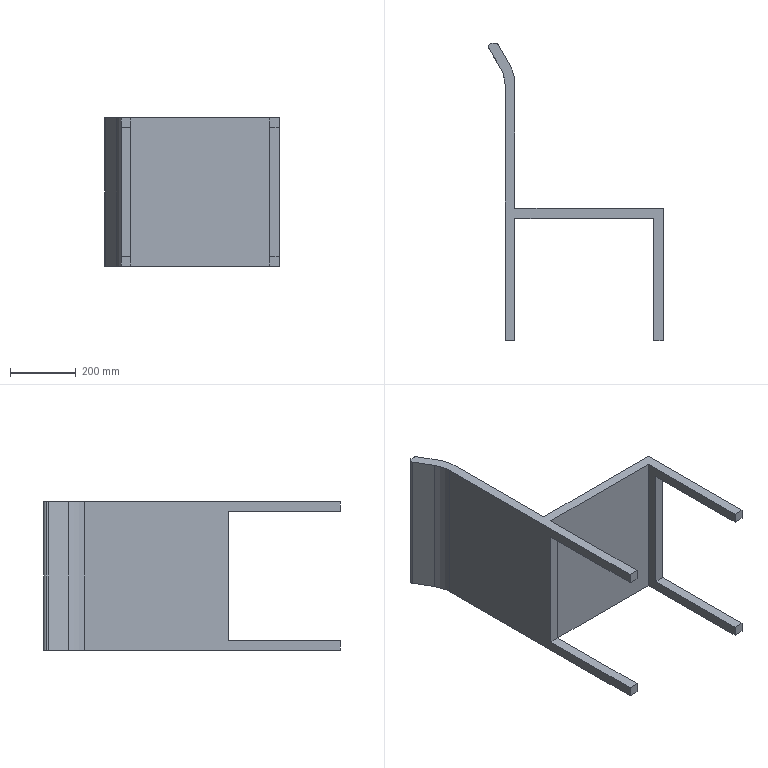Part | SolidWorks | features Extrusion 1, ICE 1 | 1 solid | 27 faces | box 529.703 x 900 x 450 mm | volume 15410155 mm3 | plane 22 | cylinder 5 | commonest cylinder face diameters 20 x3 200 x1 260 x1
STEP:
#1=CARTESIAN_POINT('',(-49.703,890.,450.));
#2=VERTEX_POINT('',#1);
#3=CARTESIAN_POINT('',(-48.352,884.98,450.));
#4=VERTEX_POINT('',#3);
#5=CARTESIAN_POINT('',(-39.703,890.,450.));
#6=DIRECTION('',(0.,0.,1.));
#7=DIRECTION('',(-1.,0.,0.));
#8=AXIS2_PLACEMENT_3D('',#5,#6,#7);
#9=CIRCLE('',#8,10.);
#10=EDGE_CURVE('',#2,#4,#9,.T.);
#11=ORIENTED_EDGE('',*,*,#10,.F.);
#12=CARTESIAN_POINT('',(-49.703,890.,0.));
#13=VERTEX_POINT('',#12);
#14=CARTESIAN_POINT('',(-49.703,890.,450.));
#15=DIRECTION('',(0.,0.,-1.));
#16=VECTOR('',#15,1000.);
#17=LINE('',#14,#16);
#18=EDGE_CURVE('',#2,#13,#17,.T.);
#19=ORIENTED_EDGE('',*,*,#18,.T.);
#20=CARTESIAN_POINT('',(-48.352,884.98,0.));
#21=VERTEX_POINT('',#20);
#22=CARTESIAN_POINT('',(-39.703,890.,0.));
#23=DIRECTION('',(0.,0.,1.));
#24=DIRECTION('',(-1.,0.,0.));
#25=AXIS2_PLACEMENT_3D('',#22,#23,#24);
#26=CIRCLE('',#25,10.);
#27=EDGE_CURVE('',#13,#21,#26,.T.);
#28=ORIENTED_EDGE('',*,*,#27,.T.);
#29=CARTESIAN_POINT('',(-48.352,884.98,450.));
#30=DIRECTION('',(0.,0.,-1.));
#31=VECTOR('',#30,1000.);
#32=LINE('',#29,#31);
#33=EDGE_CURVE('',#4,#21,#32,.T.);
#34=ORIENTED_EDGE('',*,*,#33,.F.);
#35=EDGE_LOOP('',(#11,#19,#28,#34));
#36=FACE_OUTER_BOUND('',#35,.T.);
#37=CARTESIAN_POINT('',(-39.703,890.,450.));
#38=DIRECTION('',(0.,0.,-1.));
#39=DIRECTION('',(-1.,0.,0.));
#40=AXIS2_PLACEMENT_3D('',#37,#38,#39);
#41=CYLINDRICAL_SURFACE('',#40,10.);
#42=ADVANCED_FACE('',(#36),#41,.T.);
#43=CARTESIAN_POINT('',(0.,0.,450.));
#44=VERTEX_POINT('',#43);
#45=CARTESIAN_POINT('',(0.,0.,420.));
#46=VERTEX_POINT('',#45);
#47=CARTESIAN_POINT('',(0.,0.,450.));
#48=DIRECTION('',(0.,0.,-1.));
#49=VECTOR('',#48,1000.);
#50=LINE('',#47,#49);
#51=EDGE_CURVE('',#44,#46,#50,.T.);
#52=ORIENTED_EDGE('',*,*,#51,.T.);
#53=CARTESIAN_POINT('',(30.,0.,420.));
#54=VERTEX_POINT('',#53);
#55=CARTESIAN_POINT('',(30.,0.,420.));
#56=DIRECTION('',(1.,0.,0.));
#57=VECTOR('',#56,1000.);
#58=LINE('',#55,#57);
#59=EDGE_CURVE('',#46,#54,#58,.T.);
#60=ORIENTED_EDGE('',*,*,#59,.T.);
#61=CARTESIAN_POINT('',(30.,0.,450.));
#62=VERTEX_POINT('',#61);
#63=CARTESIAN_POINT('',(30.,0.,450.));
#64=DIRECTION('',(0.,0.,-1.));
#65=VECTOR('',#64,1000.);
#66=LINE('',#63,#65);
#67=EDGE_CURVE('',#62,#54,#66,.T.);
#68=ORIENTED_EDGE('',*,*,#67,.F.);
#69=CARTESIAN_POINT('',(30.,0.,450.));
#70=DIRECTION('',(1.,0.,0.));
#71=VECTOR('',#70,1000.);
#72=LINE('',#69,#71);
#73=EDGE_CURVE('',#44,#62,#72,.T.);
#74=ORIENTED_EDGE('',*,*,#73,.F.);
#75=EDGE_LOOP('',(#52,#60,#68,#74));
#76=FACE_OUTER_BOUND('',#75,.T.);
#77=CARTESIAN_POINT('',(30.,0.,450.));
#78=DIRECTION('',(0.,1.,0.));
#79=DIRECTION('',(-1.,0.,0.));
#80=AXIS2_PLACEMENT_3D('',#77,#78,#79);
#81=PLANE('',#80);
#82=ADVANCED_FACE('',(#76),#81,.F.);
#83=CARTESIAN_POINT('',(450.,0.,450.));
#84=VERTEX_POINT('',#83);
#85=CARTESIAN_POINT('',(450.,0.,420.));
#86=VERTEX_POINT('',#85);
#87=CARTESIAN_POINT('',(450.,0.,450.));
#88=DIRECTION('',(0.,0.,-1.));
#89=VECTOR('',#88,1000.);
#90=LINE('',#87,#89);
#91=EDGE_CURVE('',#84,#86,#90,.T.);
#92=ORIENTED_EDGE('',*,*,#91,.T.);
#93=CARTESIAN_POINT('',(480.,0.,420.));
#94=VERTEX_POINT('',#93);
#95=CARTESIAN_POINT('',(480.,0.,420.));
#96=DIRECTION('',(1.,0.,0.));
#97=VECTOR('',#96,1000.);
#98=LINE('',#95,#97);
#99=EDGE_CURVE('',#86,#94,#98,.T.);
#100=ORIENTED_EDGE('',*,*,#99,.T.);
#101=CARTESIAN_POINT('',(480.,0.,450.));
#102=VERTEX_POINT('',#101);
#103=CARTESIAN_POINT('',(480.,0.,450.));
#104=DIRECTION('',(0.,0.,-1.));
#105=VECTOR('',#104,1000.);
#106=LINE('',#103,#105);
#107=EDGE_CURVE('',#102,#94,#106,.T.);
#108=ORIENTED_EDGE('',*,*,#107,.F.);
#109=CARTESIAN_POINT('',(480.,0.,450.));
#110=DIRECTION('',(1.,0.,0.));
#111=VECTOR('',#110,1000.);
#112=LINE('',#109,#111);
#113=EDGE_CURVE('',#84,#102,#112,.T.);
#114=ORIENTED_EDGE('',*,*,#113,.F.);
#115=EDGE_LOOP('',(#92,#100,#108,#114));
#116=FACE_OUTER_BOUND('',#115,.T.);
#117=CARTESIAN_POINT('',(480.,0.,450.));
#118=DIRECTION('',(0.,1.,0.));
#119=DIRECTION('',(-1.,0.,0.));
#120=AXIS2_PLACEMENT_3D('',#117,#118,#119);
#121=PLANE('',#120);
#122=ADVANCED_FACE('',(#116),#121,.F.);
#123=CARTESIAN_POINT('',(30.,0.,30.));
#124=VERTEX_POINT('',#123);
#125=CARTESIAN_POINT('',(30.,0.,0.));
#126=VERTEX_POINT('',#125);
#127=CARTESIAN_POINT('',(30.,0.,450.));
#128=DIRECTION('',(0.,0.,-1.));
#129=VECTOR('',#128,1000.);
#130=LINE('',#127,#129);
#131=EDGE_CURVE('',#124,#126,#130,.T.);
#132=ORIENTED_EDGE('',*,*,#131,.F.);
#133=CARTESIAN_POINT('',(0.,0.,30.));
#134=VERTEX_POINT('',#133);
#135=CARTESIAN_POINT('',(30.,0.,30.));
#136=DIRECTION('',(-1.,0.,0.));
#137=VECTOR('',#136,1000.);
#138=LINE('',#135,#137);
#139=EDGE_CURVE('',#124,#134,#138,.T.);
#140=ORIENTED_EDGE('',*,*,#139,.T.);
#141=CARTESIAN_POINT('',(0.,0.,0.));
#142=VERTEX_POINT('',#141);
#143=CARTESIAN_POINT('',(0.,0.,450.));
#144=DIRECTION('',(0.,0.,-1.));
#145=VECTOR('',#144,1000.);
#146=LINE('',#143,#145);
#147=EDGE_CURVE('',#134,#142,#146,.T.);
#148=ORIENTED_EDGE('',*,*,#147,.T.);
#149=CARTESIAN_POINT('',(30.,0.,0.));
#150=DIRECTION('',(1.,0.,0.));
#151=VECTOR('',#150,1000.);
#152=LINE('',#149,#151);
#153=EDGE_CURVE('',#142,#126,#152,.T.);
#154=ORIENTED_EDGE('',*,*,#153,.T.);
#155=EDGE_LOOP('',(#132,#140,#148,#154));
#156=FACE_OUTER_BOUND('',#155,.T.);
#157=CARTESIAN_POINT('',(30.,0.,450.));
#158=DIRECTION('',(0.,1.,0.));
#159=DIRECTION('',(-1.,0.,0.));
#160=AXIS2_PLACEMENT_3D('',#157,#158,#159);
#161=PLANE('',#160);
#162=ADVANCED_FACE('',(#156),#161,.F.);
#163=ORIENTED_EDGE('',*,*,#67,.T.);
#164=CARTESIAN_POINT('',(30.,340.,420.));
#165=VERTEX_POINT('',#164);
#166=CARTESIAN_POINT('',(30.,370.,420.));
#167=DIRECTION('',(0.,1.,0.));
#168=VECTOR('',#167,1000.);
#169=LINE('',#166,#168);
#170=EDGE_CURVE('',#54,#165,#169,.T.);
#171=ORIENTED_EDGE('',*,*,#170,.T.);
#172=CARTESIAN_POINT('',(30.,340.,30.));
#173=VERTEX_POINT('',#172);
#174=CARTESIAN_POINT('',(30.,340.,450.));
#175=DIRECTION('',(0.,0.,-1.));
#176=VECTOR('',#175,1000.);
#177=LINE('',#174,#176);
#178=EDGE_CURVE('',#165,#173,#177,.T.);
#179=ORIENTED_EDGE('',*,*,#178,.T.);
#180=CARTESIAN_POINT('',(30.,370.,30.));
#181=DIRECTION('',(0.,-1.,0.));
#182=VECTOR('',#181,1000.);
#183=LINE('',#180,#182);
#184=EDGE_CURVE('',#173,#124,#183,.T.);
#185=ORIENTED_EDGE('',*,*,#184,.T.);
#186=ORIENTED_EDGE('',*,*,#131,.T.);
#187=CARTESIAN_POINT('',(30.,370.,0.));
#188=VERTEX_POINT('',#187);
#189=CARTESIAN_POINT('',(30.,370.,0.));
#190=DIRECTION('',(0.,1.,0.));
#191=VECTOR('',#190,1000.);
#192=LINE('',#189,#191);
#193=EDGE_CURVE('',#126,#188,#192,.T.);
#194=ORIENTED_EDGE('',*,*,#193,.T.);
#195=CARTESIAN_POINT('',(30.,370.,450.));
#196=VERTEX_POINT('',#195);
#197=CARTESIAN_POINT('',(30.,370.,450.));
#198=DIRECTION('',(0.,0.,-1.));
#199=VECTOR('',#198,1000.);
#200=LINE('',#197,#199);
#201=EDGE_CURVE('',#196,#188,#200,.T.);
#202=ORIENTED_EDGE('',*,*,#201,.F.);
#203=CARTESIAN_POINT('',(30.,370.,450.));
#204=DIRECTION('',(0.,1.,0.));
#205=VECTOR('',#204,1000.);
#206=LINE('',#203,#205);
#207=EDGE_CURVE('',#62,#196,#206,.T.);
#208=ORIENTED_EDGE('',*,*,#207,.F.);
#209=EDGE_LOOP('',(#163,#171,#179,#185,#186,#194,#202,#208));
#210=FACE_OUTER_BOUND('',#209,.T.);
#211=CARTESIAN_POINT('',(30.,370.,450.));
#212=DIRECTION('',(-1.,0.,0.));
#213=DIRECTION('',(0.,-1.,0.));
#214=AXIS2_PLACEMENT_3D('',#211,#212,#213);
#215=PLANE('',#214);
#216=ADVANCED_FACE('',(#210),#215,.F.);
#217=CARTESIAN_POINT('',(450.,370.,0.));
#218=VERTEX_POINT('',#217);
#219=CARTESIAN_POINT('',(450.,370.,0.));
#220=DIRECTION('',(1.,0.,0.));
#221=VECTOR('',#220,1000.);
#222=LINE('',#219,#221);
#223=EDGE_CURVE('',#188,#218,#222,.T.);
#224=ORIENTED_EDGE('',*,*,#223,.T.);
#225=CARTESIAN_POINT('',(450.,370.,450.));
#226=VERTEX_POINT('',#225);
#227=CARTESIAN_POINT('',(450.,370.,450.));
#228=DIRECTION('',(0.,0.,-1.));
#229=VECTOR('',#228,1000.);
#230=LINE('',#227,#229);
#231=EDGE_CURVE('',#226,#218,#230,.T.);
#232=ORIENTED_EDGE('',*,*,#231,.F.);
#233=CARTESIAN_POINT('',(450.,370.,450.));
#234=DIRECTION('',(1.,0.,0.));
#235=VECTOR('',#234,1000.);
#236=LINE('',#233,#235);
#237=EDGE_CURVE('',#196,#226,#236,.T.);
#238=ORIENTED_EDGE('',*,*,#237,.F.);
#239=ORIENTED_EDGE('',*,*,#201,.T.);
#240=EDGE_LOOP('',(#224,#232,#238,#239));
#241=FACE_OUTER_BOUND('',#240,.T.);
#242=CARTESIAN_POINT('',(450.,370.,450.));
#243=DIRECTION('',(0.,1.,0.));
#244=DIRECTION('',(-1.,0.,0.));
#245=AXIS2_PLACEMENT_3D('',#242,#243,#244);
#246=PLANE('',#245);
#247=ADVANCED_FACE('',(#241),#246,.F.);
#248=CARTESIAN_POINT('',(450.,340.,30.));
#249=VERTEX_POINT('',#248);
#250=CARTESIAN_POINT('',(450.,340.,420.));
#251=VERTEX_POINT('',#250);
#252=CARTESIAN_POINT('',(450.,340.,450.));
#253=DIRECTION('',(0.,0.,1.));
#254=VECTOR('',#253,1000.);
#255=LINE('',#252,#254);
#256=EDGE_CURVE('',#249,#251,#255,.T.);
#257=ORIENTED_EDGE('',*,*,#256,.T.);
#258=CARTESIAN_POINT('',(450.,0.,420.));
#259=DIRECTION('',(0.,-1.,0.));
#260=VECTOR('',#259,1000.);
#261=LINE('',#258,#260);
#262=EDGE_CURVE('',#251,#86,#261,.T.);
#263=ORIENTED_EDGE('',*,*,#262,.T.);
#264=ORIENTED_EDGE('',*,*,#91,.F.);
#265=CARTESIAN_POINT('',(450.,0.,450.));
#266=DIRECTION('',(0.,-1.,0.));
#267=VECTOR('',#266,1000.);
#268=LINE('',#265,#267);
#269=EDGE_CURVE('',#226,#84,#268,.T.);
#270=ORIENTED_EDGE('',*,*,#269,.F.);
#271=ORIENTED_EDGE('',*,*,#231,.T.);
#272=CARTESIAN_POINT('',(450.,0.,0.));
#273=VERTEX_POINT('',#272);
#274=CARTESIAN_POINT('',(450.,0.,0.));
#275=DIRECTION('',(0.,-1.,0.));
#276=VECTOR('',#275,1000.);
#277=LINE('',#274,#276);
#278=EDGE_CURVE('',#218,#273,#277,.T.);
#279=ORIENTED_EDGE('',*,*,#278,.T.);
#280=CARTESIAN_POINT('',(450.,0.,30.));
#281=VERTEX_POINT('',#280);
#282=CARTESIAN_POINT('',(450.,0.,450.));
#283=DIRECTION('',(0.,0.,-1.));
#284=VECTOR('',#283,1000.);
#285=LINE('',#282,#284);
#286=EDGE_CURVE('',#281,#273,#285,.T.);
#287=ORIENTED_EDGE('',*,*,#286,.F.);
#288=CARTESIAN_POINT('',(450.,0.,30.));
#289=DIRECTION('',(0.,1.,0.));
#290=VECTOR('',#289,1000.);
#291=LINE('',#288,#290);
#292=EDGE_CURVE('',#281,#249,#291,.T.);
#293=ORIENTED_EDGE('',*,*,#292,.T.);
#294=EDGE_LOOP('',(#257,#263,#264,#270,#271,#279,#287,#293));
#295=FACE_OUTER_BOUND('',#294,.T.);
#296=CARTESIAN_POINT('',(450.,0.,450.));
#297=DIRECTION('',(1.,0.,0.));
#298=DIRECTION('',(0.,0.,-1.));
#299=AXIS2_PLACEMENT_3D('',#296,#297,#298);
#300=PLANE('',#299);
#301=ADVANCED_FACE('',(#295),#300,.F.);
#302=CARTESIAN_POINT('',(480.,0.,30.));
#303=VERTEX_POINT('',#302);
#304=CARTESIAN_POINT('',(480.,0.,0.));
#305=VERTEX_POINT('',#304);
#306=CARTESIAN_POINT('',(480.,0.,450.));
#307=DIRECTION('',(0.,0.,-1.));
#308=VECTOR('',#307,1000.);
#309=LINE('',#306,#308);
#310=EDGE_CURVE('',#303,#305,#309,.T.);
#311=ORIENTED_EDGE('',*,*,#310,.F.);
#312=CARTESIAN_POINT('',(480.,0.,30.));
#313=DIRECTION('',(-1.,0.,0.));
#314=VECTOR('',#313,1000.);
#315=LINE('',#312,#314);
#316=EDGE_CURVE('',#303,#281,#315,.T.);
#317=ORIENTED_EDGE('',*,*,#316,.T.);
#318=ORIENTED_EDGE('',*,*,#286,.T.);
#319=CARTESIAN_POINT('',(480.,0.,0.));
#320=DIRECTION('',(1.,0.,0.));
#321=VECTOR('',#320,1000.);
#322=LINE('',#319,#321);
#323=EDGE_CURVE('',#273,#305,#322,.T.);
#324=ORIENTED_EDGE('',*,*,#323,.T.);
#325=EDGE_LOOP('',(#311,#317,#318,#324));
#326=FACE_OUTER_BOUND('',#325,.T.);
#327=CARTESIAN_POINT('',(480.,0.,450.));
#328=DIRECTION('',(0.,1.,0.));
#329=DIRECTION('',(-1.,0.,0.));
#330=AXIS2_PLACEMENT_3D('',#327,#328,#329);
#331=PLANE('',#330);
#332=ADVANCED_FACE('',(#326),#331,.F.);
#333=ORIENTED_EDGE('',*,*,#107,.T.);
#334=CARTESIAN_POINT('',(480.,340.,420.));
#335=VERTEX_POINT('',#334);
#336=CARTESIAN_POINT('',(480.,340.,420.));
#337=DIRECTION('',(0.,-1.,0.));
#338=VECTOR('',#337,1000.);
#339=LINE('',#336,#338);
#340=EDGE_CURVE('',#335,#94,#339,.T.);
#341=ORIENTED_EDGE('',*,*,#340,.F.);
#342=CARTESIAN_POINT('',(480.,340.,30.));
#343=VERTEX_POINT('',#342);
#344=CARTESIAN_POINT('',(480.,340.,420.));
#345=DIRECTION('',(0.,0.,1.));
#346=VECTOR('',#345,1000.);
#347=LINE('',#344,#346);
#348=EDGE_CURVE('',#343,#335,#347,.T.);
#349=ORIENTED_EDGE('',*,*,#348,.F.);
#350=CARTESIAN_POINT('',(480.,340.,30.));
#351=DIRECTION('',(0.,1.,0.));
#352=VECTOR('',#351,1000.);
#353=LINE('',#350,#352);
#354=EDGE_CURVE('',#303,#343,#353,.T.);
#355=ORIENTED_EDGE('',*,*,#354,.F.);
#356=ORIENTED_EDGE('',*,*,#310,.T.);
#357=CARTESIAN_POINT('',(480.,400.,0.));
#358=VERTEX_POINT('',#357);
#359=CARTESIAN_POINT('',(480.,400.,0.));
#360=DIRECTION('',(0.,1.,0.));
#361=VECTOR('',#360,1000.);
#362=LINE('',#359,#361);
#363=EDGE_CURVE('',#305,#358,#362,.T.);
#364=ORIENTED_EDGE('',*,*,#363,.T.);
#365=CARTESIAN_POINT('',(480.,400.,450.));
#366=VERTEX_POINT('',#365);
#367=CARTESIAN_POINT('',(480.,400.,450.));
#368=DIRECTION('',(0.,0.,-1.));
#369=VECTOR('',#368,1000.);
#370=LINE('',#367,#369);
#371=EDGE_CURVE('',#366,#358,#370,.T.);
#372=ORIENTED_EDGE('',*,*,#371,.F.);
#373=CARTESIAN_POINT('',(480.,400.,450.));
#374=DIRECTION('',(0.,1.,0.));
#375=VECTOR('',#374,1000.);
#376=LINE('',#373,#375);
#377=EDGE_CURVE('',#102,#366,#376,.T.);
#378=ORIENTED_EDGE('',*,*,#377,.F.);
#379=EDGE_LOOP('',(#333,#341,#349,#355,#356,#364,#372,#378));
#380=FACE_OUTER_BOUND('',#379,.T.);
#381=CARTESIAN_POINT('',(480.,400.,450.));
#382=DIRECTION('',(-1.,0.,0.));
#383=DIRECTION('',(0.,-1.,0.));
#384=AXIS2_PLACEMENT_3D('',#381,#382,#383);
#385=PLANE('',#384);
#386=ADVANCED_FACE('',(#380),#385,.F.);
#387=CARTESIAN_POINT('',(30.,400.,0.));
#388=VERTEX_POINT('',#387);
#389=CARTESIAN_POINT('',(30.,400.,0.));
#390=DIRECTION('',(-1.,0.,0.));
#391=VECTOR('',#390,1000.);
#392=LINE('',#389,#391);
#393=EDGE_CURVE('',#358,#388,#392,.T.);
#394=ORIENTED_EDGE('',*,*,#393,.T.);
#395=CARTESIAN_POINT('',(30.,400.,450.));
#396=VERTEX_POINT('',#395);
#397=CARTESIAN_POINT('',(30.,400.,450.));
#398=DIRECTION('',(0.,0.,-1.));
#399=VECTOR('',#398,1000.);
#400=LINE('',#397,#399);
#401=EDGE_CURVE('',#396,#388,#400,.T.);
#402=ORIENTED_EDGE('',*,*,#401,.F.);
#403=CARTESIAN_POINT('',(30.,400.,450.));
#404=DIRECTION('',(-1.,0.,0.));
#405=VECTOR('',#404,1000.);
#406=LINE('',#403,#405);
#407=EDGE_CURVE('',#366,#396,#406,.T.);
#408=ORIENTED_EDGE('',*,*,#407,.F.);
#409=ORIENTED_EDGE('',*,*,#371,.T.);
#410=EDGE_LOOP('',(#394,#402,#408,#409));
#411=FACE_OUTER_BOUND('',#410,.T.);
#412=CARTESIAN_POINT('',(30.,400.,450.));
#413=DIRECTION('',(0.,-1.,0.));
#414=DIRECTION('',(0.,0.,-1.));
#415=AXIS2_PLACEMENT_3D('',#412,#413,#414);
#416=PLANE('',#415);
#417=ADVANCED_FACE('',(#411),#416,.F.);
#418=CARTESIAN_POINT('',(30.,774.762,0.));
#419=VERTEX_POINT('',#418);
#420=CARTESIAN_POINT('',(30.,774.762,0.));
#421=DIRECTION('',(0.,1.,0.));
#422=VECTOR('',#421,1000.);
#423=LINE('',#420,#422);
#424=EDGE_CURVE('',#388,#419,#423,.T.);
#425=ORIENTED_EDGE('',*,*,#424,.T.);
#426=CARTESIAN_POINT('',(30.,774.762,450.));
#427=VERTEX_POINT('',#426);
#428=CARTESIAN_POINT('',(30.,774.762,450.));
#429=DIRECTION('',(0.,0.,-1.));
#430=VECTOR('',#429,1000.);
#431=LINE('',#428,#430);
#432=EDGE_CURVE('',#427,#419,#431,.T.);
#433=ORIENTED_EDGE('',*,*,#432,.F.);
#434=CARTESIAN_POINT('',(30.,774.762,450.));
#435=DIRECTION('',(0.,1.,0.));
#436=VECTOR('',#435,1000.);
#437=LINE('',#434,#436);
#438=EDGE_CURVE('',#396,#427,#437,.T.);
#439=ORIENTED_EDGE('',*,*,#438,.F.);
#440=ORIENTED_EDGE('',*,*,#401,.T.);
#441=EDGE_LOOP('',(#425,#433,#439,#440));
#442=FACE_OUTER_BOUND('',#441,.T.);
#443=CARTESIAN_POINT('',(30.,774.762,450.));
#444=DIRECTION('',(-1.,0.,0.));
#445=DIRECTION('',(0.,-1.,0.));
#446=AXIS2_PLACEMENT_3D('',#443,#444,#445);
#447=PLANE('',#446);
#448=ADVANCED_FACE('',(#442),#447,.F.);
#449=CARTESIAN_POINT('',(12.431,840.025,0.));
#450=VERTEX_POINT('',#449);
#451=CARTESIAN_POINT('',(-100.,774.762,0.));
#452=DIRECTION('',(0.,0.,1.));
#453=DIRECTION('',(-1.,0.,0.));
#454=AXIS2_PLACEMENT_3D('',#451,#452,#453);
#455=CIRCLE('',#454,130.);
#456=EDGE_CURVE('',#419,#450,#455,.T.);
#457=ORIENTED_EDGE('',*,*,#456,.T.);
#458=CARTESIAN_POINT('',(12.431,840.025,450.));
#459=VERTEX_POINT('',#458);
#460=CARTESIAN_POINT('',(12.431,840.025,450.));
#461=DIRECTION('',(0.,0.,-1.));
#462=VECTOR('',#461,1000.);
#463=LINE('',#460,#462);
#464=EDGE_CURVE('',#459,#450,#463,.T.);
#465=ORIENTED_EDGE('',*,*,#464,.F.);
#466=CARTESIAN_POINT('',(-100.,774.762,450.));
#467=DIRECTION('',(0.,0.,1.));
#468=DIRECTION('',(-1.,0.,0.));
#469=AXIS2_PLACEMENT_3D('',#466,#467,#468);
#470=CIRCLE('',#469,130.);
#471=EDGE_CURVE('',#427,#459,#470,.T.);
#472=ORIENTED_EDGE('',*,*,#471,.F.);
#473=ORIENTED_EDGE('',*,*,#432,.T.);
#474=EDGE_LOOP('',(#457,#465,#472,#473));
#475=FACE_OUTER_BOUND('',#474,.T.);
#476=CARTESIAN_POINT('',(-100.,774.762,450.));
#477=DIRECTION('',(0.,0.,-1.));
#478=DIRECTION('',(-1.,0.,0.));
#479=AXIS2_PLACEMENT_3D('',#476,#477,#478);
#480=CYLINDRICAL_SURFACE('',#479,130.);
#481=ADVANCED_FACE('',(#475),#480,.T.);
#482=CARTESIAN_POINT('',(-19.492,895.02,0.));
#483=VERTEX_POINT('',#482);
#484=CARTESIAN_POINT('',(12.431,840.025,0.));
#485=DIRECTION('',(-0.502,0.8649,0.));
#486=VECTOR('',#485,1000.);
#487=LINE('',#484,#486);
#488=EDGE_CURVE('',#450,#483,#487,.T.);
#489=ORIENTED_EDGE('',*,*,#488,.T.);
#490=CARTESIAN_POINT('',(-19.492,895.02,450.));
#491=VERTEX_POINT('',#490);
#492=CARTESIAN_POINT('',(-19.492,895.02,450.));
#493=DIRECTION('',(0.,0.,-1.));
#494=VECTOR('',#493,1000.);
#495=LINE('',#492,#494);
#496=EDGE_CURVE('',#491,#483,#495,.T.);
#497=ORIENTED_EDGE('',*,*,#496,.F.);
#498=CARTESIAN_POINT('',(12.431,840.025,450.));
#499=DIRECTION('',(-0.502,0.8649,0.));
#500=VECTOR('',#499,1000.);
#501=LINE('',#498,#500);
#502=EDGE_CURVE('',#459,#491,#501,.T.);
#503=ORIENTED_EDGE('',*,*,#502,.F.);
#504=ORIENTED_EDGE('',*,*,#464,.T.);
#505=EDGE_LOOP('',(#489,#497,#503,#504));
#506=FACE_OUTER_BOUND('',#505,.T.);
#507=CARTESIAN_POINT('',(12.431,840.025,450.));
#508=DIRECTION('',(-0.8649,-0.502,0.));
#509=DIRECTION('',(0.502,-0.8649,0.));
#510=AXIS2_PLACEMENT_3D('',#507,#508,#509);
#511=PLANE('',#510);
#512=ADVANCED_FACE('',(#506),#511,.F.);
#513=CARTESIAN_POINT('',(-28.141,900.,0.));
#514=VERTEX_POINT('',#513);
#515=CARTESIAN_POINT('',(-28.141,890.,0.));
#516=DIRECTION('',(0.,0.,1.));
#517=DIRECTION('',(1.,0.,0.));
#518=AXIS2_PLACEMENT_3D('',#515,#516,#517);
#519=CIRCLE('',#518,10.);
#520=EDGE_CURVE('',#483,#514,#519,.T.);
#521=ORIENTED_EDGE('',*,*,#520,.T.);
#522=CARTESIAN_POINT('',(-28.141,900.,450.));
#523=VERTEX_POINT('',#522);
#524=CARTESIAN_POINT('',(-28.141,900.,450.));
#525=DIRECTION('',(0.,0.,-1.));
#526=VECTOR('',#525,1000.);
#527=LINE('',#524,#526);
#528=EDGE_CURVE('',#523,#514,#527,.T.);
#529=ORIENTED_EDGE('',*,*,#528,.F.);
#530=CARTESIAN_POINT('',(-28.141,890.,450.));
#531=DIRECTION('',(0.,0.,1.));
#532=DIRECTION('',(1.,0.,0.));
#533=AXIS2_PLACEMENT_3D('',#530,#531,#532);
#534=CIRCLE('',#533,10.);
#535=EDGE_CURVE('',#491,#523,#534,.T.);
#536=ORIENTED_EDGE('',*,*,#535,.F.);
#537=ORIENTED_EDGE('',*,*,#496,.T.);
#538=EDGE_LOOP('',(#521,#529,#536,#537));
#539=FACE_OUTER_BOUND('',#538,.T.);
#540=CARTESIAN_POINT('',(-28.141,890.,450.));
#541=DIRECTION('',(0.,0.,-1.));
#542=DIRECTION('',(-1.,0.,0.));
#543=AXIS2_PLACEMENT_3D('',#540,#541,#542);
#544=CYLINDRICAL_SURFACE('',#543,10.);
#545=ADVANCED_FACE('',(#539),#544,.T.);
#546=CARTESIAN_POINT('',(-39.703,900.,0.));
#547=VERTEX_POINT('',#546);
#548=CARTESIAN_POINT('',(-28.141,900.,0.));
#549=DIRECTION('',(-1.,0.,0.));
#550=VECTOR('',#549,1000.);
#551=LINE('',#548,#550);
#552=EDGE_CURVE('',#514,#547,#551,.T.);
#553=ORIENTED_EDGE('',*,*,#552,.T.);
#554=CARTESIAN_POINT('',(-39.703,900.,450.));
#555=VERTEX_POINT('',#554);
#556=CARTESIAN_POINT('',(-39.703,900.,450.));
#557=DIRECTION('',(0.,0.,-1.));
#558=VECTOR('',#557,1000.);
#559=LINE('',#556,#558);
#560=EDGE_CURVE('',#555,#547,#559,.T.);
#561=ORIENTED_EDGE('',*,*,#560,.F.);
#562=CARTESIAN_POINT('',(-28.141,900.,450.));
#563=DIRECTION('',(-1.,0.,0.));
#564=VECTOR('',#563,1000.);
#565=LINE('',#562,#564);
#566=EDGE_CURVE('',#523,#555,#565,.T.);
#567=ORIENTED_EDGE('',*,*,#566,.F.);
#568=ORIENTED_EDGE('',*,*,#528,.T.);
#569=EDGE_LOOP('',(#553,#561,#567,#568));
#570=FACE_OUTER_BOUND('',#569,.T.);
#571=CARTESIAN_POINT('',(-28.141,900.,450.));
#572=DIRECTION('',(0.,-1.,0.));
#573=DIRECTION('',(0.,0.,-1.));
#574=AXIS2_PLACEMENT_3D('',#571,#572,#573);
#575=PLANE('',#574);
#576=ADVANCED_FACE('',(#570),#575,.F.);
#577=ORIENTED_EDGE('',*,*,#18,.F.);
#578=CARTESIAN_POINT('',(-39.703,890.,450.));
#579=DIRECTION('',(0.,0.,1.));
#580=DIRECTION('',(-1.,0.,0.));
#581=AXIS2_PLACEMENT_3D('',#578,#579,#580);
#582=CIRCLE('',#581,10.);
#583=EDGE_CURVE('',#555,#2,#582,.T.);
#584=ORIENTED_EDGE('',*,*,#583,.F.);
#585=ORIENTED_EDGE('',*,*,#560,.T.);
#586=CARTESIAN_POINT('',(-39.703,890.,0.));
#587=DIRECTION('',(0.,0.,1.));
#588=DIRECTION('',(-1.,0.,0.));
#589=AXIS2_PLACEMENT_3D('',#586,#587,#588);
#590=CIRCLE('',#589,10.);
#591=EDGE_CURVE('',#547,#13,#590,.T.);
#592=ORIENTED_EDGE('',*,*,#591,.T.);
#593=EDGE_LOOP('',(#577,#584,#585,#592));
#594=FACE_OUTER_BOUND('',#593,.T.);
#595=CARTESIAN_POINT('',(-39.703,890.,450.));
#596=DIRECTION('',(0.,0.,-1.));
#597=DIRECTION('',(-1.,0.,0.));
#598=AXIS2_PLACEMENT_3D('',#595,#596,#597);
#599=CYLINDRICAL_SURFACE('',#598,10.);
#600=ADVANCED_FACE('',(#594),#599,.T.);
#601=CARTESIAN_POINT('',(-13.515,824.964,0.));
#602=VERTEX_POINT('',#601);
#603=CARTESIAN_POINT('',(-13.515,824.964,0.));
#604=DIRECTION('',(0.502,-0.8649,0.));
#605=VECTOR('',#604,1000.);
#606=LINE('',#603,#605);
#607=EDGE_CURVE('',#21,#602,#606,.T.);
#608=ORIENTED_EDGE('',*,*,#607,.T.);
#609=CARTESIAN_POINT('',(-13.515,824.964,450.));
#610=VERTEX_POINT('',#609);
#611=CARTESIAN_POINT('',(-13.515,824.964,450.));
#612=DIRECTION('',(0.,0.,-1.));
#613=VECTOR('',#612,1000.);
#614=LINE('',#611,#613);
#615=EDGE_CURVE('',#610,#602,#614,.T.);
#616=ORIENTED_EDGE('',*,*,#615,.F.);
#617=CARTESIAN_POINT('',(-13.515,824.964,450.));
#618=DIRECTION('',(0.502,-0.8649,0.));
#619=VECTOR('',#618,1000.);
#620=LINE('',#617,#619);
#621=EDGE_CURVE('',#4,#610,#620,.T.);
#622=ORIENTED_EDGE('',*,*,#621,.F.);
#623=ORIENTED_EDGE('',*,*,#33,.T.);
#624=EDGE_LOOP('',(#608,#616,#622,#623));
#625=FACE_OUTER_BOUND('',#624,.T.);
#626=CARTESIAN_POINT('',(-13.515,824.964,450.));
#627=DIRECTION('',(0.8649,0.502,0.));
#628=DIRECTION('',(-0.502,0.8649,0.));
#629=AXIS2_PLACEMENT_3D('',#626,#627,#628);
#630=PLANE('',#629);
#631=ADVANCED_FACE('',(#625),#630,.F.);
#632=CARTESIAN_POINT('',(0.,774.762,0.));
#633=VERTEX_POINT('',#632);
#634=CARTESIAN_POINT('',(-100.,774.762,0.));
#635=DIRECTION('',(0.,0.,-1.));
#636=DIRECTION('',(1.,0.,0.));
#637=AXIS2_PLACEMENT_3D('',#634,#635,#636);
#638=CIRCLE('',#637,100.);
#639=EDGE_CURVE('',#602,#633,#638,.T.);
#640=ORIENTED_EDGE('',*,*,#639,.T.);
#641=CARTESIAN_POINT('',(0.,774.762,450.));
#642=VERTEX_POINT('',#641);
#643=CARTESIAN_POINT('',(0.,774.762,450.));
#644=DIRECTION('',(0.,0.,-1.));
#645=VECTOR('',#644,1000.);
#646=LINE('',#643,#645);
#647=EDGE_CURVE('',#642,#633,#646,.T.);
#648=ORIENTED_EDGE('',*,*,#647,.F.);
#649=CARTESIAN_POINT('',(-100.,774.762,450.));
#650=DIRECTION('',(0.,0.,-1.));
#651=DIRECTION('',(1.,0.,0.));
#652=AXIS2_PLACEMENT_3D('',#649,#650,#651);
#653=CIRCLE('',#652,100.);
#654=EDGE_CURVE('',#610,#642,#653,.T.);
#655=ORIENTED_EDGE('',*,*,#654,.F.);
#656=ORIENTED_EDGE('',*,*,#615,.T.);
#657=EDGE_LOOP('',(#640,#648,#655,#656));
#658=FACE_OUTER_BOUND('',#657,.T.);
#659=CARTESIAN_POINT('',(-100.,774.762,450.));
#660=DIRECTION('',(0.,0.,-1.));
#661=DIRECTION('',(-1.,0.,0.));
#662=AXIS2_PLACEMENT_3D('',#659,#660,#661);
#663=CYLINDRICAL_SURFACE('',#662,100.);
#664=ADVANCED_FACE('',(#658),#663,.F.);
#665=CARTESIAN_POINT('',(0.,340.,30.));
#666=VERTEX_POINT('',#665);
#667=CARTESIAN_POINT('',(0.,340.,420.));
#668=VERTEX_POINT('',#667);
#669=CARTESIAN_POINT('',(0.,340.,450.));
#670=DIRECTION('',(0.,0.,1.));
#671=VECTOR('',#670,1000.);
#672=LINE('',#669,#671);
#673=EDGE_CURVE('',#666,#668,#672,.T.);
#674=ORIENTED_EDGE('',*,*,#673,.T.);
#675=CARTESIAN_POINT('',(0.,0.,420.));
#676=DIRECTION('',(0.,-1.,0.));
#677=VECTOR('',#676,1000.);
#678=LINE('',#675,#677);
#679=EDGE_CURVE('',#668,#46,#678,.T.);
#680=ORIENTED_EDGE('',*,*,#679,.T.);
#681=ORIENTED_EDGE('',*,*,#51,.F.);
#682=CARTESIAN_POINT('',(0.,0.,450.));
#683=DIRECTION('',(0.,-1.,0.));
#684=VECTOR('',#683,1000.);
#685=LINE('',#682,#684);
#686=EDGE_CURVE('',#642,#44,#685,.T.);
#687=ORIENTED_EDGE('',*,*,#686,.F.);
#688=ORIENTED_EDGE('',*,*,#647,.T.);
#689=CARTESIAN_POINT('',(0.,0.,0.));
#690=DIRECTION('',(0.,-1.,0.));
#691=VECTOR('',#690,1000.);
#692=LINE('',#689,#691);
#693=EDGE_CURVE('',#633,#142,#692,.T.);
#694=ORIENTED_EDGE('',*,*,#693,.T.);
#695=ORIENTED_EDGE('',*,*,#147,.F.);
#696=CARTESIAN_POINT('',(0.,0.,30.));
#697=DIRECTION('',(0.,1.,0.));
#698=VECTOR('',#697,1000.);
#699=LINE('',#696,#698);
#700=EDGE_CURVE('',#134,#666,#699,.T.);
#701=ORIENTED_EDGE('',*,*,#700,.T.);
#702=EDGE_LOOP('',(#674,#680,#681,#687,#688,#694,#695,#701));
#703=FACE_OUTER_BOUND('',#702,.T.);
#704=CARTESIAN_POINT('',(0.,0.,450.));
#705=DIRECTION('',(1.,0.,0.));
#706=DIRECTION('',(0.,1.,0.));
#707=AXIS2_PLACEMENT_3D('',#704,#705,#706);
#708=PLANE('',#707);
#709=ADVANCED_FACE('',(#703),#708,.F.);
#710=ORIENTED_EDGE('',*,*,#73,.T.);
#711=ORIENTED_EDGE('',*,*,#207,.T.);
#712=ORIENTED_EDGE('',*,*,#237,.T.);
#713=ORIENTED_EDGE('',*,*,#269,.T.);
#714=ORIENTED_EDGE('',*,*,#113,.T.);
#715=ORIENTED_EDGE('',*,*,#377,.T.);
#716=ORIENTED_EDGE('',*,*,#407,.T.);
#717=ORIENTED_EDGE('',*,*,#438,.T.);
#718=ORIENTED_EDGE('',*,*,#471,.T.);
#719=ORIENTED_EDGE('',*,*,#502,.T.);
#720=ORIENTED_EDGE('',*,*,#535,.T.);
#721=ORIENTED_EDGE('',*,*,#566,.T.);
#722=ORIENTED_EDGE('',*,*,#583,.T.);
#723=ORIENTED_EDGE('',*,*,#10,.T.);
#724=ORIENTED_EDGE('',*,*,#621,.T.);
#725=ORIENTED_EDGE('',*,*,#654,.T.);
#726=ORIENTED_EDGE('',*,*,#686,.T.);
#727=EDGE_LOOP('',(#710,#711,#712,#713,#714,#715,#716,#717,#718,#719,#720,#721,#722,#723,#724,#725,#726));
#728=FACE_OUTER_BOUND('',#727,.T.);
#729=CARTESIAN_POINT('',(-100.,774.762,450.));
#730=DIRECTION('',(0.,0.,1.));
#731=DIRECTION('',(1.,0.,0.));
#732=AXIS2_PLACEMENT_3D('',#729,#730,#731);
#733=PLANE('',#732);
#734=ADVANCED_FACE('',(#728),#733,.T.);
#735=ORIENTED_EDGE('',*,*,#153,.F.);
#736=ORIENTED_EDGE('',*,*,#693,.F.);
#737=ORIENTED_EDGE('',*,*,#639,.F.);
#738=ORIENTED_EDGE('',*,*,#607,.F.);
#739=ORIENTED_EDGE('',*,*,#27,.F.);
#740=ORIENTED_EDGE('',*,*,#591,.F.);
#741=ORIENTED_EDGE('',*,*,#552,.F.);
#742=ORIENTED_EDGE('',*,*,#520,.F.);
#743=ORIENTED_EDGE('',*,*,#488,.F.);
#744=ORIENTED_EDGE('',*,*,#456,.F.);
#745=ORIENTED_EDGE('',*,*,#424,.F.);
#746=ORIENTED_EDGE('',*,*,#393,.F.);
#747=ORIENTED_EDGE('',*,*,#363,.F.);
#748=ORIENTED_EDGE('',*,*,#323,.F.);
#749=ORIENTED_EDGE('',*,*,#278,.F.);
#750=ORIENTED_EDGE('',*,*,#223,.F.);
#751=ORIENTED_EDGE('',*,*,#193,.F.);
#752=EDGE_LOOP('',(#735,#736,#737,#738,#739,#740,#741,#742,#743,#744,#745,#746,#747,#748,#749,#750,#751));
#753=FACE_OUTER_BOUND('',#752,.T.);
#754=CARTESIAN_POINT('',(-100.,774.762,0.));
#755=DIRECTION('',(0.,0.,1.));
#756=DIRECTION('',(1.,0.,0.));
#757=AXIS2_PLACEMENT_3D('',#754,#755,#756);
#758=PLANE('',#757);
#759=ADVANCED_FACE('',(#753),#758,.F.);
#760=CARTESIAN_POINT('',(-20.,340.,30.));
#761=DIRECTION('',(1.,0.,0.));
#762=VECTOR('',#761,1000.);
#763=LINE('',#760,#762);
#764=EDGE_CURVE('',#666,#173,#763,.T.);
#765=ORIENTED_EDGE('',*,*,#764,.F.);
#766=ORIENTED_EDGE('',*,*,#700,.F.);
#767=ORIENTED_EDGE('',*,*,#139,.F.);
#768=ORIENTED_EDGE('',*,*,#184,.F.);
#769=EDGE_LOOP('',(#765,#766,#767,#768));
#770=FACE_OUTER_BOUND('',#769,.T.);
#771=CARTESIAN_POINT('',(-20.,340.,30.));
#772=DIRECTION('',(0.,0.,-1.));
#773=DIRECTION('',(0.,1.,0.));
#774=AXIS2_PLACEMENT_3D('',#771,#772,#773);
#775=PLANE('',#774);
#776=ADVANCED_FACE('',(#770),#775,.F.);
#777=CARTESIAN_POINT('',(-20.,340.,420.));
#778=DIRECTION('',(1.,0.,0.));
#779=VECTOR('',#778,1000.);
#780=LINE('',#777,#779);
#781=EDGE_CURVE('',#668,#165,#780,.T.);
#782=ORIENTED_EDGE('',*,*,#781,.F.);
#783=ORIENTED_EDGE('',*,*,#673,.F.);
#784=ORIENTED_EDGE('',*,*,#764,.T.);
#785=ORIENTED_EDGE('',*,*,#178,.F.);
#786=EDGE_LOOP('',(#782,#783,#784,#785));
#787=FACE_OUTER_BOUND('',#786,.T.);
#788=CARTESIAN_POINT('',(-20.,340.,420.));
#789=DIRECTION('',(0.,1.,0.));
#790=DIRECTION('',(-1.,0.,0.));
#791=AXIS2_PLACEMENT_3D('',#788,#789,#790);
#792=PLANE('',#791);
#793=ADVANCED_FACE('',(#787),#792,.F.);
#794=ORIENTED_EDGE('',*,*,#59,.F.);
#795=ORIENTED_EDGE('',*,*,#679,.F.);
#796=ORIENTED_EDGE('',*,*,#781,.T.);
#797=ORIENTED_EDGE('',*,*,#170,.F.);
#798=EDGE_LOOP('',(#794,#795,#796,#797));
#799=FACE_OUTER_BOUND('',#798,.T.);
#800=CARTESIAN_POINT('',(-20.,340.,420.));
#801=DIRECTION('',(0.,0.,1.));
#802=DIRECTION('',(1.,0.,0.));
#803=AXIS2_PLACEMENT_3D('',#800,#801,#802);
#804=PLANE('',#803);
#805=ADVANCED_FACE('',(#799),#804,.F.);
#806=CARTESIAN_POINT('',(-20.,340.,420.));
#807=DIRECTION('',(1.,0.,0.));
#808=VECTOR('',#807,1000.);
#809=LINE('',#806,#808);
#810=EDGE_CURVE('',#251,#335,#809,.T.);
#811=ORIENTED_EDGE('',*,*,#810,.T.);
#812=ORIENTED_EDGE('',*,*,#340,.T.);
#813=ORIENTED_EDGE('',*,*,#99,.F.);
#814=ORIENTED_EDGE('',*,*,#262,.F.);
#815=EDGE_LOOP('',(#811,#812,#813,#814));
#816=FACE_OUTER_BOUND('',#815,.T.);
#817=CARTESIAN_POINT('',(-20.,340.,420.));
#818=DIRECTION('',(0.,0.,1.));
#819=DIRECTION('',(1.,0.,0.));
#820=AXIS2_PLACEMENT_3D('',#817,#818,#819);
#821=PLANE('',#820);
#822=ADVANCED_FACE('',(#816),#821,.F.);
#823=CARTESIAN_POINT('',(-20.,340.,30.));
#824=DIRECTION('',(1.,0.,0.));
#825=VECTOR('',#824,1000.);
#826=LINE('',#823,#825);
#827=EDGE_CURVE('',#249,#343,#826,.T.);
#828=ORIENTED_EDGE('',*,*,#827,.T.);
#829=ORIENTED_EDGE('',*,*,#348,.T.);
#830=ORIENTED_EDGE('',*,*,#810,.F.);
#831=ORIENTED_EDGE('',*,*,#256,.F.);
#832=EDGE_LOOP('',(#828,#829,#830,#831));
#833=FACE_OUTER_BOUND('',#832,.T.);
#834=CARTESIAN_POINT('',(-20.,340.,420.));
#835=DIRECTION('',(0.,1.,0.));
#836=DIRECTION('',(-1.,0.,0.));
#837=AXIS2_PLACEMENT_3D('',#834,#835,#836);
#838=PLANE('',#837);
#839=ADVANCED_FACE('',(#833),#838,.F.);
#840=ORIENTED_EDGE('',*,*,#316,.F.);
#841=ORIENTED_EDGE('',*,*,#354,.T.);
#842=ORIENTED_EDGE('',*,*,#827,.F.);
#843=ORIENTED_EDGE('',*,*,#292,.F.);
#844=EDGE_LOOP('',(#840,#841,#842,#843));
#845=FACE_OUTER_BOUND('',#844,.T.);
#846=CARTESIAN_POINT('',(-20.,340.,30.));
#847=DIRECTION('',(0.,0.,-1.));
#848=DIRECTION('',(0.,1.,0.));
#849=AXIS2_PLACEMENT_3D('',#846,#847,#848);
#850=PLANE('',#849);
#851=ADVANCED_FACE('',(#845),#850,.F.);
#852=CLOSED_SHELL('',(#42,#82,#122,#162,#216,#247,#301,#332,#386,#417,#448,#481,#512,#545,#576,#600,#631,#664,#709,#734,#759,#776,#793,#805,#822,#839,#851));
#853=MANIFOLD_SOLID_BREP('',#852);
#854=CARTESIAN_POINT('',(0.,0.,0.));
#855=DIRECTION('',(0.,0.,1.));
#856=DIRECTION('',(1.,0.,0.));
#857=AXIS2_PLACEMENT_3D('',#854,#855,#856);
#858=(LENGTH_UNIT()NAMED_UNIT(*)SI_UNIT(.MILLI.,.METRE.));
#859=UNCERTAINTY_MEASURE_WITH_UNIT(LENGTH_MEASURE(0.00001),#858,'','');
#860=(NAMED_UNIT(*)PLANE_ANGLE_UNIT()SI_UNIT($,.RADIAN.));
#861=(NAMED_UNIT(*)SI_UNIT($,.STERADIAN.)SOLID_ANGLE_UNIT());
#862=(GEOMETRIC_REPRESENTATION_CONTEXT(3)GLOBAL_UNCERTAINTY_ASSIGNED_CONTEXT((#859))GLOBAL_UNIT_ASSIGNED_CONTEXT((#858,#860,#861))REPRESENTATION_CONTEXT('',''));
#863=ADVANCED_BREP_SHAPE_REPRESENTATION('',(#853,#857),#862);